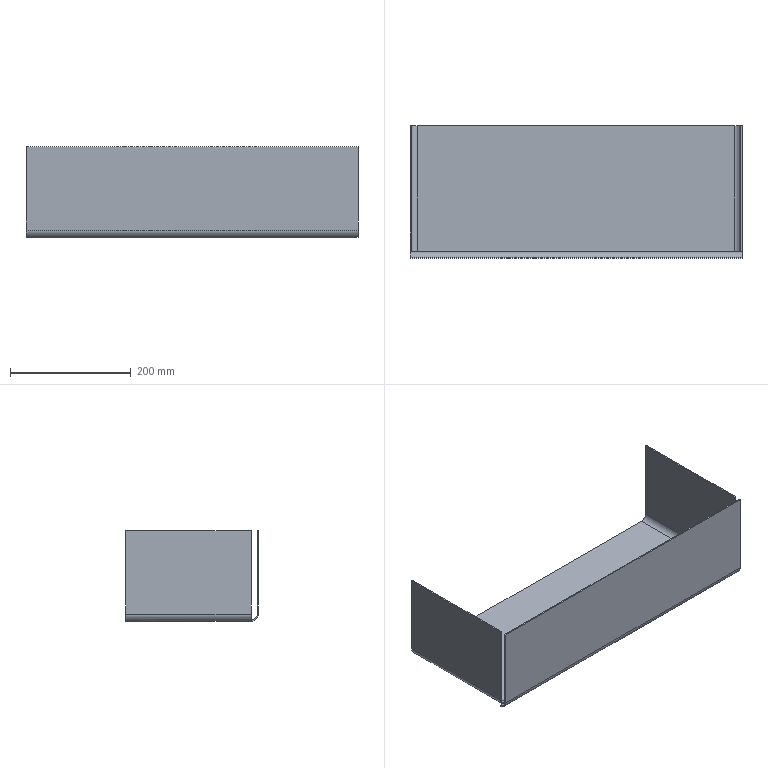Part | STEP file | MYT-A01-P25 | 1 solid | 32 faces | box 550 x 220 x 150 mm | volume 518815 mm3 | plane 26 | cylinder 6 | commonest cylinder face diameters 20 x3 24 x3
STEP:
#1=CARTESIAN_POINT('',(-275.,-98.,2.));
#2=VERTEX_POINT('',#1);
#3=CARTESIAN_POINT('',(-269.633,-98.,2.));
#4=VERTEX_POINT('',#3);
#5=CARTESIAN_POINT('',(-275.,-98.,2.));
#6=DIRECTION('',(1.,0.,0.));
#7=VECTOR('',#6,1000.);
#8=LINE('',#5,#7);
#9=EDGE_CURVE('',#2,#4,#8,.T.);
#10=ORIENTED_EDGE('',*,*,#9,.T.);
#11=CARTESIAN_POINT('',(-263.,-98.,0.));
#12=VERTEX_POINT('',#11);
#13=CARTESIAN_POINT('',(-263.,-98.,12.));
#14=DIRECTION('',(0.,-1.,0.));
#15=DIRECTION('',(0.,0.,-1.));
#16=AXIS2_PLACEMENT_3D('',#13,#14,#15);
#17=CIRCLE('',#16,12.);
#18=EDGE_CURVE('',#4,#12,#17,.T.);
#19=ORIENTED_EDGE('',*,*,#18,.T.);
#20=CARTESIAN_POINT('',(-275.,-98.,0.));
#21=VERTEX_POINT('',#20);
#22=CARTESIAN_POINT('',(275.,-98.,0.));
#23=DIRECTION('',(1.,0.,0.));
#24=VECTOR('',#23,1000.);
#25=LINE('',#22,#24);
#26=EDGE_CURVE('',#21,#12,#25,.T.);
#27=ORIENTED_EDGE('',*,*,#26,.F.);
#28=CARTESIAN_POINT('',(-275.,-98.,2.));
#29=DIRECTION('',(0.,0.,-1.));
#30=VECTOR('',#29,1000.);
#31=LINE('',#28,#30);
#32=EDGE_CURVE('',#2,#21,#31,.T.);
#33=ORIENTED_EDGE('',*,*,#32,.F.);
#34=EDGE_LOOP('',(#10,#19,#27,#33));
#35=FACE_OUTER_BOUND('',#34,.T.);
#36=CARTESIAN_POINT('',(-275.,-98.,2.));
#37=DIRECTION('',(0.,1.,0.));
#38=DIRECTION('',(0.,0.,1.));
#39=AXIS2_PLACEMENT_3D('',#36,#37,#38);
#40=PLANE('',#39);
#41=ADVANCED_FACE('',(#35),#40,.T.);
#42=CARTESIAN_POINT('',(275.,-98.,0.));
#43=VERTEX_POINT('',#42);
#44=CARTESIAN_POINT('',(263.,-98.,0.));
#45=VERTEX_POINT('',#44);
#46=CARTESIAN_POINT('',(275.,-98.,0.));
#47=DIRECTION('',(-1.,0.,0.));
#48=VECTOR('',#47,1000.);
#49=LINE('',#46,#48);
#50=EDGE_CURVE('',#43,#45,#49,.T.);
#51=ORIENTED_EDGE('',*,*,#50,.T.);
#52=CARTESIAN_POINT('',(269.633,-98.,2.));
#53=VERTEX_POINT('',#52);
#54=CARTESIAN_POINT('',(263.,-98.,12.));
#55=DIRECTION('',(0.,-1.,0.));
#56=DIRECTION('',(0.,0.,1.));
#57=AXIS2_PLACEMENT_3D('',#54,#55,#56);
#58=CIRCLE('',#57,12.);
#59=EDGE_CURVE('',#45,#53,#58,.T.);
#60=ORIENTED_EDGE('',*,*,#59,.T.);
#61=CARTESIAN_POINT('',(275.,-98.,2.));
#62=VERTEX_POINT('',#61);
#63=CARTESIAN_POINT('',(275.,-98.,2.));
#64=DIRECTION('',(-1.,0.,0.));
#65=VECTOR('',#64,1000.);
#66=LINE('',#63,#65);
#67=EDGE_CURVE('',#62,#53,#66,.T.);
#68=ORIENTED_EDGE('',*,*,#67,.F.);
#69=CARTESIAN_POINT('',(275.,-98.,2.));
#70=DIRECTION('',(0.,0.,-1.));
#71=VECTOR('',#70,1000.);
#72=LINE('',#69,#71);
#73=EDGE_CURVE('',#62,#43,#72,.T.);
#74=ORIENTED_EDGE('',*,*,#73,.T.);
#75=EDGE_LOOP('',(#51,#60,#68,#74));
#76=FACE_OUTER_BOUND('',#75,.T.);
#77=CARTESIAN_POINT('',(263.,-98.,2.));
#78=DIRECTION('',(0.,1.,0.));
#79=DIRECTION('',(0.,0.,1.));
#80=AXIS2_PLACEMENT_3D('',#77,#78,#79);
#81=PLANE('',#80);
#82=ADVANCED_FACE('',(#76),#81,.T.);
#83=CARTESIAN_POINT('',(263.,110.,2.));
#84=VERTEX_POINT('',#83);
#85=CARTESIAN_POINT('',(-263.,110.,2.));
#86=VERTEX_POINT('',#85);
#87=CARTESIAN_POINT('',(-275.,110.,2.));
#88=DIRECTION('',(-1.,0.,0.));
#89=VECTOR('',#88,1000.);
#90=LINE('',#87,#89);
#91=EDGE_CURVE('',#84,#86,#90,.T.);
#92=ORIENTED_EDGE('',*,*,#91,.T.);
#93=CARTESIAN_POINT('',(-263.,-98.,2.));
#94=VERTEX_POINT('',#93);
#95=CARTESIAN_POINT('',(-263.,-98.,2.));
#96=DIRECTION('',(0.,1.,0.));
#97=VECTOR('',#96,1000.);
#98=LINE('',#95,#97);
#99=EDGE_CURVE('',#94,#86,#98,.T.);
#100=ORIENTED_EDGE('',*,*,#99,.F.);
#101=CARTESIAN_POINT('',(263.,-98.,2.));
#102=VERTEX_POINT('',#101);
#103=CARTESIAN_POINT('',(275.,-98.,2.));
#104=DIRECTION('',(-1.,0.,0.));
#105=VECTOR('',#104,1000.);
#106=LINE('',#103,#105);
#107=EDGE_CURVE('',#102,#94,#106,.T.);
#108=ORIENTED_EDGE('',*,*,#107,.F.);
#109=CARTESIAN_POINT('',(263.,110.,2.));
#110=DIRECTION('',(0.,-1.,0.));
#111=VECTOR('',#110,1000.);
#112=LINE('',#109,#111);
#113=EDGE_CURVE('',#84,#102,#112,.T.);
#114=ORIENTED_EDGE('',*,*,#113,.F.);
#115=EDGE_LOOP('',(#92,#100,#108,#114));
#116=FACE_OUTER_BOUND('',#115,.T.);
#117=CARTESIAN_POINT('',(0.,0.,2.));
#118=DIRECTION('',(0.,0.,1.));
#119=DIRECTION('',(1.,0.,0.));
#120=AXIS2_PLACEMENT_3D('',#117,#118,#119);
#121=PLANE('',#120);
#122=ADVANCED_FACE('',(#116),#121,.T.);
#123=CARTESIAN_POINT('',(-263.,110.,0.));
#124=VERTEX_POINT('',#123);
#125=CARTESIAN_POINT('',(-263.,-98.,0.));
#126=DIRECTION('',(0.,1.,0.));
#127=VECTOR('',#126,1000.);
#128=LINE('',#125,#127);
#129=EDGE_CURVE('',#12,#124,#128,.T.);
#130=ORIENTED_EDGE('',*,*,#129,.T.);
#131=CARTESIAN_POINT('',(263.,110.,0.));
#132=VERTEX_POINT('',#131);
#133=CARTESIAN_POINT('',(0.,110.,0.));
#134=DIRECTION('',(-1.,0.,0.));
#135=VECTOR('',#134,1000.);
#136=LINE('',#133,#135);
#137=EDGE_CURVE('',#132,#124,#136,.T.);
#138=ORIENTED_EDGE('',*,*,#137,.F.);
#139=CARTESIAN_POINT('',(263.,110.,0.));
#140=DIRECTION('',(0.,-1.,0.));
#141=VECTOR('',#140,1000.);
#142=LINE('',#139,#141);
#143=EDGE_CURVE('',#132,#45,#142,.T.);
#144=ORIENTED_EDGE('',*,*,#143,.T.);
#145=CARTESIAN_POINT('',(275.,-98.,0.));
#146=DIRECTION('',(-1.,0.,0.));
#147=VECTOR('',#146,1000.);
#148=LINE('',#145,#147);
#149=EDGE_CURVE('',#45,#12,#148,.T.);
#150=ORIENTED_EDGE('',*,*,#149,.T.);
#151=EDGE_LOOP('',(#130,#138,#144,#150));
#152=FACE_OUTER_BOUND('',#151,.T.);
#153=CARTESIAN_POINT('',(0.,0.,0.));
#154=DIRECTION('',(0.,0.,1.));
#155=DIRECTION('',(1.,0.,0.));
#156=AXIS2_PLACEMENT_3D('',#153,#154,#155);
#157=PLANE('',#156);
#158=ADVANCED_FACE('',(#152),#157,.F.);
#159=CARTESIAN_POINT('',(-263.,110.,2.));
#160=DIRECTION('',(0.,0.,-1.));
#161=VECTOR('',#160,1000.);
#162=LINE('',#159,#161);
#163=EDGE_CURVE('',#86,#124,#162,.T.);
#164=ORIENTED_EDGE('',*,*,#163,.F.);
#165=ORIENTED_EDGE('',*,*,#91,.F.);
#166=CARTESIAN_POINT('',(263.,110.,2.));
#167=DIRECTION('',(0.,0.,-1.));
#168=VECTOR('',#167,1000.);
#169=LINE('',#166,#168);
#170=EDGE_CURVE('',#84,#132,#169,.T.);
#171=ORIENTED_EDGE('',*,*,#170,.T.);
#172=ORIENTED_EDGE('',*,*,#137,.T.);
#173=EDGE_LOOP('',(#164,#165,#171,#172));
#174=FACE_OUTER_BOUND('',#173,.T.);
#175=CARTESIAN_POINT('',(-275.,110.,2.));
#176=DIRECTION('',(0.,1.,0.));
#177=DIRECTION('',(-1.,0.,0.));
#178=AXIS2_PLACEMENT_3D('',#175,#176,#177);
#179=PLANE('',#178);
#180=ADVANCED_FACE('',(#174),#179,.T.);
#181=CARTESIAN_POINT('',(-275.,-108.,12.));
#182=VERTEX_POINT('',#181);
#183=CARTESIAN_POINT('',(-275.,-110.,12.));
#184=VERTEX_POINT('',#183);
#185=CARTESIAN_POINT('',(-275.,-110.,12.));
#186=DIRECTION('',(0.,-1.,0.));
#187=VECTOR('',#186,1000.);
#188=LINE('',#185,#187);
#189=EDGE_CURVE('',#182,#184,#188,.T.);
#190=ORIENTED_EDGE('',*,*,#189,.F.);
#191=CARTESIAN_POINT('',(-275.,-98.,12.));
#192=DIRECTION('',(-1.,0.,0.));
#193=DIRECTION('',(0.,0.,-1.));
#194=AXIS2_PLACEMENT_3D('',#191,#192,#193);
#195=CIRCLE('',#194,10.);
#196=EDGE_CURVE('',#2,#182,#195,.T.);
#197=ORIENTED_EDGE('',*,*,#196,.F.);
#198=ORIENTED_EDGE('',*,*,#32,.T.);
#199=CARTESIAN_POINT('',(-275.,-98.,12.));
#200=DIRECTION('',(-1.,0.,0.));
#201=DIRECTION('',(0.,0.,-1.));
#202=AXIS2_PLACEMENT_3D('',#199,#200,#201);
#203=CIRCLE('',#202,12.);
#204=EDGE_CURVE('',#21,#184,#203,.T.);
#205=ORIENTED_EDGE('',*,*,#204,.T.);
#206=EDGE_LOOP('',(#190,#197,#198,#205));
#207=FACE_OUTER_BOUND('',#206,.T.);
#208=CARTESIAN_POINT('',(-275.,-98.,12.));
#209=DIRECTION('',(-1.,0.,0.));
#210=DIRECTION('',(0.,0.,1.));
#211=AXIS2_PLACEMENT_3D('',#208,#209,#210);
#212=PLANE('',#211);
#213=ADVANCED_FACE('',(#207),#212,.T.);
#214=CARTESIAN_POINT('',(275.,-108.,12.));
#215=VERTEX_POINT('',#214);
#216=CARTESIAN_POINT('',(275.,-98.,12.));
#217=DIRECTION('',(1.,0.,0.));
#218=DIRECTION('',(0.,0.,-1.));
#219=AXIS2_PLACEMENT_3D('',#216,#217,#218);
#220=CIRCLE('',#219,10.);
#221=EDGE_CURVE('',#215,#62,#220,.T.);
#222=ORIENTED_EDGE('',*,*,#221,.F.);
#223=CARTESIAN_POINT('',(275.,-110.,12.));
#224=VERTEX_POINT('',#223);
#225=CARTESIAN_POINT('',(275.,-108.,12.));
#226=DIRECTION('',(0.,-1.,0.));
#227=VECTOR('',#226,1000.);
#228=LINE('',#225,#227);
#229=EDGE_CURVE('',#215,#224,#228,.T.);
#230=ORIENTED_EDGE('',*,*,#229,.T.);
#231=CARTESIAN_POINT('',(275.,-98.,12.));
#232=DIRECTION('',(1.,0.,0.));
#233=DIRECTION('',(0.,0.,-1.));
#234=AXIS2_PLACEMENT_3D('',#231,#232,#233);
#235=CIRCLE('',#234,12.);
#236=EDGE_CURVE('',#224,#43,#235,.T.);
#237=ORIENTED_EDGE('',*,*,#236,.T.);
#238=ORIENTED_EDGE('',*,*,#73,.F.);
#239=EDGE_LOOP('',(#222,#230,#237,#238));
#240=FACE_OUTER_BOUND('',#239,.T.);
#241=CARTESIAN_POINT('',(275.,-98.,12.));
#242=DIRECTION('',(-1.,0.,0.));
#243=DIRECTION('',(0.,0.,1.));
#244=AXIS2_PLACEMENT_3D('',#241,#242,#243);
#245=PLANE('',#244);
#246=ADVANCED_FACE('',(#240),#245,.F.);
#247=ORIENTED_EDGE('',*,*,#50,.F.);
#248=ORIENTED_EDGE('',*,*,#236,.F.);
#249=CARTESIAN_POINT('',(-275.,-110.,12.));
#250=DIRECTION('',(-1.,0.,0.));
#251=VECTOR('',#250,1000.);
#252=LINE('',#249,#251);
#253=EDGE_CURVE('',#224,#184,#252,.T.);
#254=ORIENTED_EDGE('',*,*,#253,.T.);
#255=ORIENTED_EDGE('',*,*,#204,.F.);
#256=ORIENTED_EDGE('',*,*,#26,.T.);
#257=ORIENTED_EDGE('',*,*,#149,.F.);
#258=EDGE_LOOP('',(#247,#248,#254,#255,#256,#257));
#259=FACE_OUTER_BOUND('',#258,.T.);
#260=CARTESIAN_POINT('',(275.,-98.,12.));
#261=DIRECTION('',(1.,0.,0.));
#262=DIRECTION('',(0.,-1.,0.));
#263=AXIS2_PLACEMENT_3D('',#260,#261,#262);
#264=CYLINDRICAL_SURFACE('',#263,12.);
#265=ADVANCED_FACE('',(#259),#264,.T.);
#266=ORIENTED_EDGE('',*,*,#67,.T.);
#267=CARTESIAN_POINT('',(275.,-98.,2.));
#268=DIRECTION('',(-1.,0.,0.));
#269=VECTOR('',#268,1000.);
#270=LINE('',#267,#269);
#271=EDGE_CURVE('',#53,#102,#270,.T.);
#272=ORIENTED_EDGE('',*,*,#271,.T.);
#273=ORIENTED_EDGE('',*,*,#107,.T.);
#274=CARTESIAN_POINT('',(-275.,-98.,2.));
#275=DIRECTION('',(1.,0.,0.));
#276=VECTOR('',#275,1000.);
#277=LINE('',#274,#276);
#278=EDGE_CURVE('',#4,#94,#277,.T.);
#279=ORIENTED_EDGE('',*,*,#278,.F.);
#280=ORIENTED_EDGE('',*,*,#9,.F.);
#281=ORIENTED_EDGE('',*,*,#196,.T.);
#282=CARTESIAN_POINT('',(-275.,-108.,12.));
#283=DIRECTION('',(1.,0.,0.));
#284=VECTOR('',#283,1000.);
#285=LINE('',#282,#284);
#286=EDGE_CURVE('',#182,#215,#285,.T.);
#287=ORIENTED_EDGE('',*,*,#286,.T.);
#288=ORIENTED_EDGE('',*,*,#221,.T.);
#289=EDGE_LOOP('',(#266,#272,#273,#279,#280,#281,#287,#288));
#290=FACE_OUTER_BOUND('',#289,.T.);
#291=CARTESIAN_POINT('',(275.,-98.,12.));
#292=DIRECTION('',(1.,0.,0.));
#293=DIRECTION('',(0.,-1.,0.));
#294=AXIS2_PLACEMENT_3D('',#291,#292,#293);
#295=CYLINDRICAL_SURFACE('',#294,10.);
#296=ADVANCED_FACE('',(#290),#295,.F.);
#297=ORIENTED_EDGE('',*,*,#189,.T.);
#298=CARTESIAN_POINT('',(-275.,-110.,150.));
#299=VERTEX_POINT('',#298);
#300=CARTESIAN_POINT('',(-275.,-110.,0.));
#301=DIRECTION('',(0.,0.,-1.));
#302=VECTOR('',#301,1000.);
#303=LINE('',#300,#302);
#304=EDGE_CURVE('',#299,#184,#303,.T.);
#305=ORIENTED_EDGE('',*,*,#304,.F.);
#306=CARTESIAN_POINT('',(-275.,-108.,150.));
#307=VERTEX_POINT('',#306);
#308=CARTESIAN_POINT('',(-275.,-110.,150.));
#309=DIRECTION('',(0.,1.,0.));
#310=VECTOR('',#309,1000.);
#311=LINE('',#308,#310);
#312=EDGE_CURVE('',#299,#307,#311,.T.);
#313=ORIENTED_EDGE('',*,*,#312,.T.);
#314=CARTESIAN_POINT('',(-275.,-108.,2.));
#315=DIRECTION('',(0.,0.,-1.));
#316=VECTOR('',#315,1000.);
#317=LINE('',#314,#316);
#318=EDGE_CURVE('',#307,#182,#317,.T.);
#319=ORIENTED_EDGE('',*,*,#318,.T.);
#320=EDGE_LOOP('',(#297,#305,#313,#319));
#321=FACE_OUTER_BOUND('',#320,.T.);
#322=CARTESIAN_POINT('',(-275.,-110.,2.));
#323=DIRECTION('',(1.,0.,0.));
#324=DIRECTION('',(0.,0.,-1.));
#325=AXIS2_PLACEMENT_3D('',#322,#323,#324);
#326=PLANE('',#325);
#327=ADVANCED_FACE('',(#321),#326,.F.);
#328=ORIENTED_EDGE('',*,*,#229,.F.);
#329=CARTESIAN_POINT('',(275.,-108.,150.));
#330=VERTEX_POINT('',#329);
#331=CARTESIAN_POINT('',(275.,-108.,150.));
#332=DIRECTION('',(0.,0.,1.));
#333=VECTOR('',#332,1000.);
#334=LINE('',#331,#333);
#335=EDGE_CURVE('',#215,#330,#334,.T.);
#336=ORIENTED_EDGE('',*,*,#335,.T.);
#337=CARTESIAN_POINT('',(275.,-110.,150.));
#338=VERTEX_POINT('',#337);
#339=CARTESIAN_POINT('',(275.,-110.,150.));
#340=DIRECTION('',(0.,1.,0.));
#341=VECTOR('',#340,1000.);
#342=LINE('',#339,#341);
#343=EDGE_CURVE('',#338,#330,#342,.T.);
#344=ORIENTED_EDGE('',*,*,#343,.F.);
#345=CARTESIAN_POINT('',(275.,-110.,0.));
#346=DIRECTION('',(0.,0.,1.));
#347=VECTOR('',#346,1000.);
#348=LINE('',#345,#347);
#349=EDGE_CURVE('',#224,#338,#348,.T.);
#350=ORIENTED_EDGE('',*,*,#349,.F.);
#351=EDGE_LOOP('',(#328,#336,#344,#350));
#352=FACE_OUTER_BOUND('',#351,.T.);
#353=CARTESIAN_POINT('',(275.,-110.,150.));
#354=DIRECTION('',(-1.,0.,0.));
#355=DIRECTION('',(0.,0.,1.));
#356=AXIS2_PLACEMENT_3D('',#353,#354,#355);
#357=PLANE('',#356);
#358=ADVANCED_FACE('',(#352),#357,.F.);
#359=ORIENTED_EDGE('',*,*,#253,.F.);
#360=ORIENTED_EDGE('',*,*,#349,.T.);
#361=CARTESIAN_POINT('',(0.,-110.,150.));
#362=DIRECTION('',(-1.,0.,0.));
#363=VECTOR('',#362,1000.);
#364=LINE('',#361,#363);
#365=EDGE_CURVE('',#338,#299,#364,.T.);
#366=ORIENTED_EDGE('',*,*,#365,.T.);
#367=ORIENTED_EDGE('',*,*,#304,.T.);
#368=EDGE_LOOP('',(#359,#360,#366,#367));
#369=FACE_OUTER_BOUND('',#368,.T.);
#370=CARTESIAN_POINT('',(0.,-110.,0.));
#371=DIRECTION('',(0.,1.,0.));
#372=DIRECTION('',(0.,0.,1.));
#373=AXIS2_PLACEMENT_3D('',#370,#371,#372);
#374=PLANE('',#373);
#375=ADVANCED_FACE('',(#369),#374,.F.);
#376=ORIENTED_EDGE('',*,*,#335,.F.);
#377=ORIENTED_EDGE('',*,*,#286,.F.);
#378=ORIENTED_EDGE('',*,*,#318,.F.);
#379=CARTESIAN_POINT('',(-275.,-108.,150.));
#380=DIRECTION('',(-1.,0.,0.));
#381=VECTOR('',#380,1000.);
#382=LINE('',#379,#381);
#383=EDGE_CURVE('',#330,#307,#382,.T.);
#384=ORIENTED_EDGE('',*,*,#383,.F.);
#385=EDGE_LOOP('',(#376,#377,#378,#384));
#386=FACE_OUTER_BOUND('',#385,.T.);
#387=CARTESIAN_POINT('',(0.,-108.,0.));
#388=DIRECTION('',(0.,1.,0.));
#389=DIRECTION('',(0.,0.,1.));
#390=AXIS2_PLACEMENT_3D('',#387,#388,#389);
#391=PLANE('',#390);
#392=ADVANCED_FACE('',(#386),#391,.T.);
#393=ORIENTED_EDGE('',*,*,#383,.T.);
#394=ORIENTED_EDGE('',*,*,#312,.F.);
#395=ORIENTED_EDGE('',*,*,#365,.F.);
#396=ORIENTED_EDGE('',*,*,#343,.T.);
#397=EDGE_LOOP('',(#393,#394,#395,#396));
#398=FACE_OUTER_BOUND('',#397,.T.);
#399=CARTESIAN_POINT('',(-275.,-110.,150.));
#400=DIRECTION('',(0.,0.,-1.));
#401=DIRECTION('',(0.,1.,0.));
#402=AXIS2_PLACEMENT_3D('',#399,#400,#401);
#403=PLANE('',#402);
#404=ADVANCED_FACE('',(#398),#403,.F.);
#405=ORIENTED_EDGE('',*,*,#271,.F.);
#406=CARTESIAN_POINT('',(275.,-98.,12.));
#407=VERTEX_POINT('',#406);
#408=CARTESIAN_POINT('',(263.,-98.,12.));
#409=DIRECTION('',(0.,-1.,0.));
#410=DIRECTION('',(0.,0.,1.));
#411=AXIS2_PLACEMENT_3D('',#408,#409,#410);
#412=CIRCLE('',#411,12.);
#413=EDGE_CURVE('',#53,#407,#412,.T.);
#414=ORIENTED_EDGE('',*,*,#413,.T.);
#415=CARTESIAN_POINT('',(273.,-98.,12.));
#416=VERTEX_POINT('',#415);
#417=CARTESIAN_POINT('',(275.,-98.,12.));
#418=DIRECTION('',(1.,0.,0.));
#419=VECTOR('',#418,1000.);
#420=LINE('',#417,#419);
#421=EDGE_CURVE('',#416,#407,#420,.T.);
#422=ORIENTED_EDGE('',*,*,#421,.F.);
#423=CARTESIAN_POINT('',(263.,-98.,12.));
#424=DIRECTION('',(0.,-1.,0.));
#425=DIRECTION('',(0.,0.,1.));
#426=AXIS2_PLACEMENT_3D('',#423,#424,#425);
#427=CIRCLE('',#426,10.);
#428=EDGE_CURVE('',#102,#416,#427,.T.);
#429=ORIENTED_EDGE('',*,*,#428,.F.);
#430=EDGE_LOOP('',(#405,#414,#422,#429));
#431=FACE_OUTER_BOUND('',#430,.T.);
#432=CARTESIAN_POINT('',(263.,-98.,12.));
#433=DIRECTION('',(0.,-1.,0.));
#434=DIRECTION('',(0.,0.,-1.));
#435=AXIS2_PLACEMENT_3D('',#432,#433,#434);
#436=PLANE('',#435);
#437=ADVANCED_FACE('',(#431),#436,.T.);
#438=CARTESIAN_POINT('',(273.,110.,12.));
#439=VERTEX_POINT('',#438);
#440=CARTESIAN_POINT('',(263.,110.,12.));
#441=DIRECTION('',(0.,1.,0.));
#442=DIRECTION('',(0.,0.,1.));
#443=AXIS2_PLACEMENT_3D('',#440,#441,#442);
#444=CIRCLE('',#443,10.);
#445=EDGE_CURVE('',#439,#84,#444,.T.);
#446=ORIENTED_EDGE('',*,*,#445,.F.);
#447=CARTESIAN_POINT('',(275.,110.,12.));
#448=VERTEX_POINT('',#447);
#449=CARTESIAN_POINT('',(273.,110.,12.));
#450=DIRECTION('',(1.,0.,0.));
#451=VECTOR('',#450,1000.);
#452=LINE('',#449,#451);
#453=EDGE_CURVE('',#439,#448,#452,.T.);
#454=ORIENTED_EDGE('',*,*,#453,.T.);
#455=CARTESIAN_POINT('',(263.,110.,12.));
#456=DIRECTION('',(0.,1.,0.));
#457=DIRECTION('',(0.,0.,1.));
#458=AXIS2_PLACEMENT_3D('',#455,#456,#457);
#459=CIRCLE('',#458,12.);
#460=EDGE_CURVE('',#448,#132,#459,.T.);
#461=ORIENTED_EDGE('',*,*,#460,.T.);
#462=ORIENTED_EDGE('',*,*,#170,.F.);
#463=EDGE_LOOP('',(#446,#454,#461,#462));
#464=FACE_OUTER_BOUND('',#463,.T.);
#465=CARTESIAN_POINT('',(263.,110.,12.));
#466=DIRECTION('',(0.,-1.,0.));
#467=DIRECTION('',(0.,0.,-1.));
#468=AXIS2_PLACEMENT_3D('',#465,#466,#467);
#469=PLANE('',#468);
#470=ADVANCED_FACE('',(#464),#469,.F.);
#471=ORIENTED_EDGE('',*,*,#143,.F.);
#472=ORIENTED_EDGE('',*,*,#460,.F.);
#473=CARTESIAN_POINT('',(275.,-98.,12.));
#474=DIRECTION('',(0.,-1.,0.));
#475=VECTOR('',#474,1000.);
#476=LINE('',#473,#475);
#477=EDGE_CURVE('',#448,#407,#476,.T.);
#478=ORIENTED_EDGE('',*,*,#477,.T.);
#479=ORIENTED_EDGE('',*,*,#413,.F.);
#480=ORIENTED_EDGE('',*,*,#59,.F.);
#481=EDGE_LOOP('',(#471,#472,#478,#479,#480));
#482=FACE_OUTER_BOUND('',#481,.T.);
#483=CARTESIAN_POINT('',(263.,110.,12.));
#484=DIRECTION('',(0.,1.,0.));
#485=DIRECTION('',(1.,0.,0.));
#486=AXIS2_PLACEMENT_3D('',#483,#484,#485);
#487=CYLINDRICAL_SURFACE('',#486,12.);
#488=ADVANCED_FACE('',(#482),#487,.T.);
#489=ORIENTED_EDGE('',*,*,#113,.T.);
#490=ORIENTED_EDGE('',*,*,#428,.T.);
#491=CARTESIAN_POINT('',(273.,-98.,12.));
#492=DIRECTION('',(0.,1.,0.));
#493=VECTOR('',#492,1000.);
#494=LINE('',#491,#493);
#495=EDGE_CURVE('',#416,#439,#494,.T.);
#496=ORIENTED_EDGE('',*,*,#495,.T.);
#497=ORIENTED_EDGE('',*,*,#445,.T.);
#498=EDGE_LOOP('',(#489,#490,#496,#497));
#499=FACE_OUTER_BOUND('',#498,.T.);
#500=CARTESIAN_POINT('',(263.,110.,12.));
#501=DIRECTION('',(0.,1.,0.));
#502=DIRECTION('',(1.,0.,0.));
#503=AXIS2_PLACEMENT_3D('',#500,#501,#502);
#504=CYLINDRICAL_SURFACE('',#503,10.);
#505=ADVANCED_FACE('',(#499),#504,.F.);
#506=ORIENTED_EDGE('',*,*,#421,.T.);
#507=CARTESIAN_POINT('',(275.,-98.,150.));
#508=VERTEX_POINT('',#507);
#509=CARTESIAN_POINT('',(275.,-98.,0.));
#510=DIRECTION('',(0.,0.,-1.));
#511=VECTOR('',#510,1000.);
#512=LINE('',#509,#511);
#513=EDGE_CURVE('',#508,#407,#512,.T.);
#514=ORIENTED_EDGE('',*,*,#513,.F.);
#515=CARTESIAN_POINT('',(273.,-98.,150.));
#516=VERTEX_POINT('',#515);
#517=CARTESIAN_POINT('',(275.,-98.,150.));
#518=DIRECTION('',(-1.,0.,0.));
#519=VECTOR('',#518,1000.);
#520=LINE('',#517,#519);
#521=EDGE_CURVE('',#508,#516,#520,.T.);
#522=ORIENTED_EDGE('',*,*,#521,.T.);
#523=CARTESIAN_POINT('',(273.,-98.,2.));
#524=DIRECTION('',(0.,0.,-1.));
#525=VECTOR('',#524,1000.);
#526=LINE('',#523,#525);
#527=EDGE_CURVE('',#516,#416,#526,.T.);
#528=ORIENTED_EDGE('',*,*,#527,.T.);
#529=EDGE_LOOP('',(#506,#514,#522,#528));
#530=FACE_OUTER_BOUND('',#529,.T.);
#531=CARTESIAN_POINT('',(275.,-98.,2.));
#532=DIRECTION('',(0.,1.,0.));
#533=DIRECTION('',(0.,0.,1.));
#534=AXIS2_PLACEMENT_3D('',#531,#532,#533);
#535=PLANE('',#534);
#536=ADVANCED_FACE('',(#530),#535,.F.);
#537=ORIENTED_EDGE('',*,*,#453,.F.);
#538=CARTESIAN_POINT('',(273.,110.,150.));
#539=VERTEX_POINT('',#538);
#540=CARTESIAN_POINT('',(273.,110.,150.));
#541=DIRECTION('',(0.,0.,1.));
#542=VECTOR('',#541,1000.);
#543=LINE('',#540,#542);
#544=EDGE_CURVE('',#439,#539,#543,.T.);
#545=ORIENTED_EDGE('',*,*,#544,.T.);
#546=CARTESIAN_POINT('',(275.,110.,150.));
#547=VERTEX_POINT('',#546);
#548=CARTESIAN_POINT('',(275.,110.,150.));
#549=DIRECTION('',(-1.,0.,0.));
#550=VECTOR('',#549,1000.);
#551=LINE('',#548,#550);
#552=EDGE_CURVE('',#547,#539,#551,.T.);
#553=ORIENTED_EDGE('',*,*,#552,.F.);
#554=CARTESIAN_POINT('',(275.,110.,0.));
#555=DIRECTION('',(0.,0.,1.));
#556=VECTOR('',#555,1000.);
#557=LINE('',#554,#556);
#558=EDGE_CURVE('',#448,#547,#557,.T.);
#559=ORIENTED_EDGE('',*,*,#558,.F.);
#560=EDGE_LOOP('',(#537,#545,#553,#559));
#561=FACE_OUTER_BOUND('',#560,.T.);
#562=CARTESIAN_POINT('',(275.,110.,150.));
#563=DIRECTION('',(0.,-1.,0.));
#564=DIRECTION('',(0.,0.,-1.));
#565=AXIS2_PLACEMENT_3D('',#562,#563,#564);
#566=PLANE('',#565);
#567=ADVANCED_FACE('',(#561),#566,.F.);
#568=ORIENTED_EDGE('',*,*,#477,.F.);
#569=ORIENTED_EDGE('',*,*,#558,.T.);
#570=CARTESIAN_POINT('',(275.,0.,150.));
#571=DIRECTION('',(0.,-1.,0.));
#572=VECTOR('',#571,1000.);
#573=LINE('',#570,#572);
#574=EDGE_CURVE('',#547,#508,#573,.T.);
#575=ORIENTED_EDGE('',*,*,#574,.T.);
#576=ORIENTED_EDGE('',*,*,#513,.T.);
#577=EDGE_LOOP('',(#568,#569,#575,#576));
#578=FACE_OUTER_BOUND('',#577,.T.);
#579=CARTESIAN_POINT('',(275.,0.,0.));
#580=DIRECTION('',(-1.,0.,0.));
#581=DIRECTION('',(0.,0.,1.));
#582=AXIS2_PLACEMENT_3D('',#579,#580,#581);
#583=PLANE('',#582);
#584=ADVANCED_FACE('',(#578),#583,.F.);
#585=ORIENTED_EDGE('',*,*,#544,.F.);
#586=ORIENTED_EDGE('',*,*,#495,.F.);
#587=ORIENTED_EDGE('',*,*,#527,.F.);
#588=CARTESIAN_POINT('',(273.,-98.,150.));
#589=DIRECTION('',(0.,-1.,0.));
#590=VECTOR('',#589,1000.);
#591=LINE('',#588,#590);
#592=EDGE_CURVE('',#539,#516,#591,.T.);
#593=ORIENTED_EDGE('',*,*,#592,.F.);
#594=EDGE_LOOP('',(#585,#586,#587,#593));
#595=FACE_OUTER_BOUND('',#594,.T.);
#596=CARTESIAN_POINT('',(273.,0.,0.));
#597=DIRECTION('',(-1.,0.,0.));
#598=DIRECTION('',(0.,0.,1.));
#599=AXIS2_PLACEMENT_3D('',#596,#597,#598);
#600=PLANE('',#599);
#601=ADVANCED_FACE('',(#595),#600,.T.);
#602=ORIENTED_EDGE('',*,*,#592,.T.);
#603=ORIENTED_EDGE('',*,*,#521,.F.);
#604=ORIENTED_EDGE('',*,*,#574,.F.);
#605=ORIENTED_EDGE('',*,*,#552,.T.);
#606=EDGE_LOOP('',(#602,#603,#604,#605));
#607=FACE_OUTER_BOUND('',#606,.T.);
#608=CARTESIAN_POINT('',(275.,-98.,150.));
#609=DIRECTION('',(0.,0.,-1.));
#610=DIRECTION('',(-1.,0.,0.));
#611=AXIS2_PLACEMENT_3D('',#608,#609,#610);
#612=PLANE('',#611);
#613=ADVANCED_FACE('',(#607),#612,.F.);
#614=CARTESIAN_POINT('',(-273.,110.,12.));
#615=VERTEX_POINT('',#614);
#616=CARTESIAN_POINT('',(-275.,110.,12.));
#617=VERTEX_POINT('',#616);
#618=CARTESIAN_POINT('',(-275.,110.,12.));
#619=DIRECTION('',(-1.,0.,0.));
#620=VECTOR('',#619,1000.);
#621=LINE('',#618,#620);
#622=EDGE_CURVE('',#615,#617,#621,.T.);
#623=ORIENTED_EDGE('',*,*,#622,.F.);
#624=CARTESIAN_POINT('',(-263.,110.,12.));
#625=DIRECTION('',(0.,1.,0.));
#626=DIRECTION('',(0.,0.,-1.));
#627=AXIS2_PLACEMENT_3D('',#624,#625,#626);
#628=CIRCLE('',#627,10.);
#629=EDGE_CURVE('',#86,#615,#628,.T.);
#630=ORIENTED_EDGE('',*,*,#629,.F.);
#631=ORIENTED_EDGE('',*,*,#163,.T.);
#632=CARTESIAN_POINT('',(-263.,110.,12.));
#633=DIRECTION('',(0.,1.,0.));
#634=DIRECTION('',(0.,0.,-1.));
#635=AXIS2_PLACEMENT_3D('',#632,#633,#634);
#636=CIRCLE('',#635,12.);
#637=EDGE_CURVE('',#124,#617,#636,.T.);
#638=ORIENTED_EDGE('',*,*,#637,.T.);
#639=EDGE_LOOP('',(#623,#630,#631,#638));
#640=FACE_OUTER_BOUND('',#639,.T.);
#641=CARTESIAN_POINT('',(-263.,110.,12.));
#642=DIRECTION('',(0.,1.,0.));
#643=DIRECTION('',(0.,0.,1.));
#644=AXIS2_PLACEMENT_3D('',#641,#642,#643);
#645=PLANE('',#644);
#646=ADVANCED_FACE('',(#640),#645,.T.);
#647=CARTESIAN_POINT('',(-275.,-98.,12.));
#648=VERTEX_POINT('',#647);
#649=CARTESIAN_POINT('',(-263.,-98.,12.));
#650=DIRECTION('',(0.,-1.,0.));
#651=DIRECTION('',(0.,0.,-1.));
#652=AXIS2_PLACEMENT_3D('',#649,#650,#651);
#653=CIRCLE('',#652,12.);
#654=EDGE_CURVE('',#648,#4,#653,.T.);
#655=ORIENTED_EDGE('',*,*,#654,.T.);
#656=ORIENTED_EDGE('',*,*,#278,.T.);
#657=CARTESIAN_POINT('',(-273.,-98.,12.));
#658=VERTEX_POINT('',#657);
#659=CARTESIAN_POINT('',(-263.,-98.,12.));
#660=DIRECTION('',(0.,-1.,0.));
#661=DIRECTION('',(0.,0.,-1.));
#662=AXIS2_PLACEMENT_3D('',#659,#660,#661);
#663=CIRCLE('',#662,10.);
#664=EDGE_CURVE('',#658,#94,#663,.T.);
#665=ORIENTED_EDGE('',*,*,#664,.F.);
#666=CARTESIAN_POINT('',(-273.,-98.,12.));
#667=DIRECTION('',(-1.,0.,0.));
#668=VECTOR('',#667,1000.);
#669=LINE('',#666,#668);
#670=EDGE_CURVE('',#658,#648,#669,.T.);
#671=ORIENTED_EDGE('',*,*,#670,.T.);
#672=EDGE_LOOP('',(#655,#656,#665,#671));
#673=FACE_OUTER_BOUND('',#672,.T.);
#674=CARTESIAN_POINT('',(-263.,-98.,12.));
#675=DIRECTION('',(0.,1.,0.));
#676=DIRECTION('',(0.,0.,1.));
#677=AXIS2_PLACEMENT_3D('',#674,#675,#676);
#678=PLANE('',#677);
#679=ADVANCED_FACE('',(#673),#678,.F.);
#680=ORIENTED_EDGE('',*,*,#129,.F.);
#681=ORIENTED_EDGE('',*,*,#18,.F.);
#682=ORIENTED_EDGE('',*,*,#654,.F.);
#683=CARTESIAN_POINT('',(-275.,110.,12.));
#684=DIRECTION('',(0.,1.,0.));
#685=VECTOR('',#684,1000.);
#686=LINE('',#683,#685);
#687=EDGE_CURVE('',#648,#617,#686,.T.);
#688=ORIENTED_EDGE('',*,*,#687,.T.);
#689=ORIENTED_EDGE('',*,*,#637,.F.);
#690=EDGE_LOOP('',(#680,#681,#682,#688,#689));
#691=FACE_OUTER_BOUND('',#690,.T.);
#692=CARTESIAN_POINT('',(-263.,-98.,12.));
#693=DIRECTION('',(0.,-1.,0.));
#694=DIRECTION('',(-1.,0.,0.));
#695=AXIS2_PLACEMENT_3D('',#692,#693,#694);
#696=CYLINDRICAL_SURFACE('',#695,12.);
#697=ADVANCED_FACE('',(#691),#696,.T.);
#698=ORIENTED_EDGE('',*,*,#99,.T.);
#699=ORIENTED_EDGE('',*,*,#629,.T.);
#700=CARTESIAN_POINT('',(-273.,110.,12.));
#701=DIRECTION('',(0.,-1.,0.));
#702=VECTOR('',#701,1000.);
#703=LINE('',#700,#702);
#704=EDGE_CURVE('',#615,#658,#703,.T.);
#705=ORIENTED_EDGE('',*,*,#704,.T.);
#706=ORIENTED_EDGE('',*,*,#664,.T.);
#707=EDGE_LOOP('',(#698,#699,#705,#706));
#708=FACE_OUTER_BOUND('',#707,.T.);
#709=CARTESIAN_POINT('',(-263.,-98.,12.));
#710=DIRECTION('',(0.,-1.,0.));
#711=DIRECTION('',(-1.,0.,0.));
#712=AXIS2_PLACEMENT_3D('',#709,#710,#711);
#713=CYLINDRICAL_SURFACE('',#712,10.);
#714=ADVANCED_FACE('',(#708),#713,.F.);
#715=ORIENTED_EDGE('',*,*,#622,.T.);
#716=CARTESIAN_POINT('',(-275.,110.,150.));
#717=VERTEX_POINT('',#716);
#718=CARTESIAN_POINT('',(-275.,110.,0.));
#719=DIRECTION('',(0.,0.,-1.));
#720=VECTOR('',#719,1000.);
#721=LINE('',#718,#720);
#722=EDGE_CURVE('',#717,#617,#721,.T.);
#723=ORIENTED_EDGE('',*,*,#722,.F.);
#724=CARTESIAN_POINT('',(-273.,110.,150.));
#725=VERTEX_POINT('',#724);
#726=CARTESIAN_POINT('',(-275.,110.,150.));
#727=DIRECTION('',(1.,0.,0.));
#728=VECTOR('',#727,1000.);
#729=LINE('',#726,#728);
#730=EDGE_CURVE('',#717,#725,#729,.T.);
#731=ORIENTED_EDGE('',*,*,#730,.T.);
#732=CARTESIAN_POINT('',(-273.,110.,2.));
#733=DIRECTION('',(0.,0.,-1.));
#734=VECTOR('',#733,1000.);
#735=LINE('',#732,#734);
#736=EDGE_CURVE('',#725,#615,#735,.T.);
#737=ORIENTED_EDGE('',*,*,#736,.T.);
#738=EDGE_LOOP('',(#715,#723,#731,#737));
#739=FACE_OUTER_BOUND('',#738,.T.);
#740=CARTESIAN_POINT('',(-275.,110.,2.));
#741=DIRECTION('',(0.,-1.,0.));
#742=DIRECTION('',(1.,0.,0.));
#743=AXIS2_PLACEMENT_3D('',#740,#741,#742);
#744=PLANE('',#743);
#745=ADVANCED_FACE('',(#739),#744,.F.);
#746=ORIENTED_EDGE('',*,*,#670,.F.);
#747=CARTESIAN_POINT('',(-273.,-98.,150.));
#748=VERTEX_POINT('',#747);
#749=CARTESIAN_POINT('',(-273.,-98.,150.));
#750=DIRECTION('',(0.,0.,1.));
#751=VECTOR('',#750,1000.);
#752=LINE('',#749,#751);
#753=EDGE_CURVE('',#658,#748,#752,.T.);
#754=ORIENTED_EDGE('',*,*,#753,.T.);
#755=CARTESIAN_POINT('',(-275.,-98.,150.));
#756=VERTEX_POINT('',#755);
#757=CARTESIAN_POINT('',(-275.,-98.,150.));
#758=DIRECTION('',(1.,0.,0.));
#759=VECTOR('',#758,1000.);
#760=LINE('',#757,#759);
#761=EDGE_CURVE('',#756,#748,#760,.T.);
#762=ORIENTED_EDGE('',*,*,#761,.F.);
#763=CARTESIAN_POINT('',(-275.,-98.,0.));
#764=DIRECTION('',(0.,0.,1.));
#765=VECTOR('',#764,1000.);
#766=LINE('',#763,#765);
#767=EDGE_CURVE('',#648,#756,#766,.T.);
#768=ORIENTED_EDGE('',*,*,#767,.F.);
#769=EDGE_LOOP('',(#746,#754,#762,#768));
#770=FACE_OUTER_BOUND('',#769,.T.);
#771=CARTESIAN_POINT('',(-275.,-98.,150.));
#772=DIRECTION('',(0.,1.,0.));
#773=DIRECTION('',(-1.,0.,0.));
#774=AXIS2_PLACEMENT_3D('',#771,#772,#773);
#775=PLANE('',#774);
#776=ADVANCED_FACE('',(#770),#775,.F.);
#777=ORIENTED_EDGE('',*,*,#687,.F.);
#778=ORIENTED_EDGE('',*,*,#767,.T.);
#779=CARTESIAN_POINT('',(-275.,0.,150.));
#780=DIRECTION('',(0.,1.,0.));
#781=VECTOR('',#780,1000.);
#782=LINE('',#779,#781);
#783=EDGE_CURVE('',#756,#717,#782,.T.);
#784=ORIENTED_EDGE('',*,*,#783,.T.);
#785=ORIENTED_EDGE('',*,*,#722,.T.);
#786=EDGE_LOOP('',(#777,#778,#784,#785));
#787=FACE_OUTER_BOUND('',#786,.T.);
#788=CARTESIAN_POINT('',(-275.,0.,0.));
#789=DIRECTION('',(1.,0.,0.));
#790=DIRECTION('',(0.,0.,-1.));
#791=AXIS2_PLACEMENT_3D('',#788,#789,#790);
#792=PLANE('',#791);
#793=ADVANCED_FACE('',(#787),#792,.F.);
#794=ORIENTED_EDGE('',*,*,#753,.F.);
#795=ORIENTED_EDGE('',*,*,#704,.F.);
#796=ORIENTED_EDGE('',*,*,#736,.F.);
#797=CARTESIAN_POINT('',(-273.,110.,150.));
#798=DIRECTION('',(0.,1.,0.));
#799=VECTOR('',#798,1000.);
#800=LINE('',#797,#799);
#801=EDGE_CURVE('',#748,#725,#800,.T.);
#802=ORIENTED_EDGE('',*,*,#801,.F.);
#803=EDGE_LOOP('',(#794,#795,#796,#802));
#804=FACE_OUTER_BOUND('',#803,.T.);
#805=CARTESIAN_POINT('',(-273.,0.,0.));
#806=DIRECTION('',(1.,0.,0.));
#807=DIRECTION('',(0.,0.,-1.));
#808=AXIS2_PLACEMENT_3D('',#805,#806,#807);
#809=PLANE('',#808);
#810=ADVANCED_FACE('',(#804),#809,.T.);
#811=ORIENTED_EDGE('',*,*,#801,.T.);
#812=ORIENTED_EDGE('',*,*,#730,.F.);
#813=ORIENTED_EDGE('',*,*,#783,.F.);
#814=ORIENTED_EDGE('',*,*,#761,.T.);
#815=EDGE_LOOP('',(#811,#812,#813,#814));
#816=FACE_OUTER_BOUND('',#815,.T.);
#817=CARTESIAN_POINT('',(-275.,110.,150.));
#818=DIRECTION('',(0.,0.,-1.));
#819=DIRECTION('',(-1.,0.,0.));
#820=AXIS2_PLACEMENT_3D('',#817,#818,#819);
#821=PLANE('',#820);
#822=ADVANCED_FACE('',(#816),#821,.F.);
#823=CLOSED_SHELL('',(#41,#82,#122,#158,#180,#213,#246,#265,#296,#327,#358,#375,#392,#404,#437,#470,#488,#505,#536,#567,#584,#601,#613,#646,#679,#697,#714,#745,#776,#793,#810,#822));
#824=MANIFOLD_SOLID_BREP('',#823);
#825=CARTESIAN_POINT('',(0.,0.,0.));
#826=DIRECTION('',(0.,0.,1.));
#827=DIRECTION('',(1.,0.,0.));
#828=AXIS2_PLACEMENT_3D('',#825,#826,#827);
#829=(LENGTH_UNIT()NAMED_UNIT(*)SI_UNIT(.MILLI.,.METRE.));
#830=UNCERTAINTY_MEASURE_WITH_UNIT(LENGTH_MEASURE(0.00001),#829,'','');
#831=(NAMED_UNIT(*)PLANE_ANGLE_UNIT()SI_UNIT($,.RADIAN.));
#832=(NAMED_UNIT(*)SI_UNIT($,.STERADIAN.)SOLID_ANGLE_UNIT());
#833=(GEOMETRIC_REPRESENTATION_CONTEXT(3)GLOBAL_UNCERTAINTY_ASSIGNED_CONTEXT((#830))GLOBAL_UNIT_ASSIGNED_CONTEXT((#829,#831,#832))REPRESENTATION_CONTEXT('',''));
#834=ADVANCED_BREP_SHAPE_REPRESENTATION('',(#824,#828),#833);